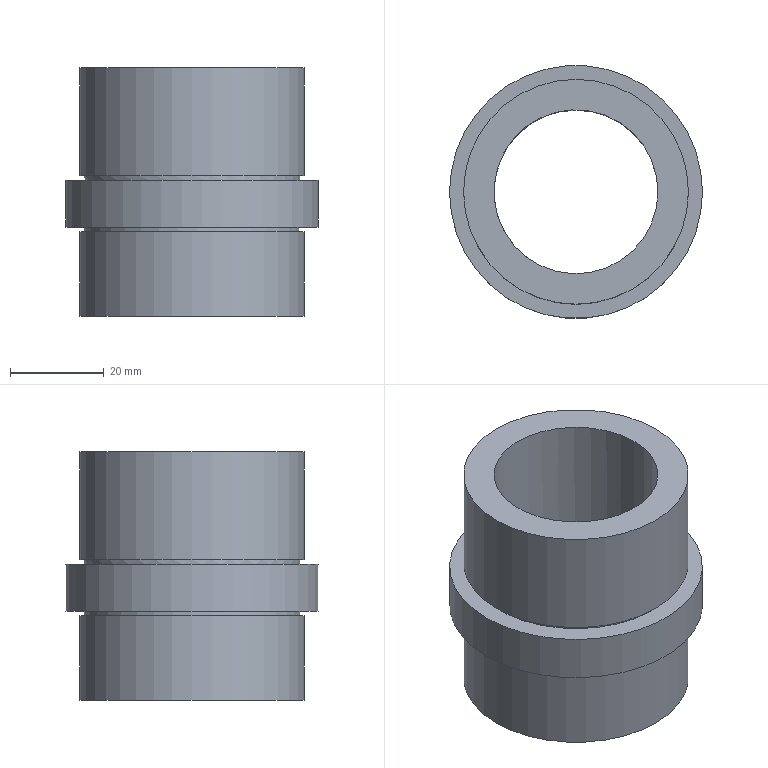Part | STEP file | 车灯-后视镜_id30_x_t | 1 solid | 12 faces | box 54 x 54 x 53 mm | volume 49426 mm3 | cylinder 6 | plane 6 | commonest cylinder face diameters 46 x2 48 x2 35 x1 54 x1
STEP:
#1=CARTESIAN_POINT('',(86.,185.,-254.5));
#2=VERTEX_POINT('',#1);
#3=CARTESIAN_POINT('',(110.,185.,-254.5));
#4=DIRECTION('',(0.,0.,1.));
#5=DIRECTION('',(-1.,0.,0.));
#6=AXIS2_PLACEMENT_3D('',#3,#4,#5);
#7=CIRCLE('',#6,24.);
#8=EDGE_CURVE('',#2,#2,#7,.T.);
#9=ORIENTED_EDGE('',*,*,#8,.T.);
#10=EDGE_LOOP('',(#9));
#11=FACE_BOUND('',#10,.T.);
#12=CARTESIAN_POINT('',(86.,185.,-231.5));
#13=VERTEX_POINT('',#12);
#14=CARTESIAN_POINT('',(110.,185.,-231.5));
#15=DIRECTION('',(0.,0.,1.));
#16=DIRECTION('',(-1.,0.,0.));
#17=AXIS2_PLACEMENT_3D('',#14,#15,#16);
#18=CIRCLE('',#17,24.);
#19=EDGE_CURVE('',#13,#13,#18,.T.);
#20=ORIENTED_EDGE('',*,*,#19,.F.);
#21=EDGE_LOOP('',(#20));
#22=FACE_BOUND('',#21,.T.);
#23=CARTESIAN_POINT('',(110.,185.,-284.5));
#24=DIRECTION('',(0.,0.,1.));
#25=DIRECTION('',(1.,0.,0.));
#26=AXIS2_PLACEMENT_3D('',#23,#24,#25);
#27=CYLINDRICAL_SURFACE('',#26,24.);
#28=ADVANCED_FACE('',(#11,#22),#27,.T.);
#29=CARTESIAN_POINT('',(127.5,185.,-231.5));
#30=VERTEX_POINT('',#29);
#31=CARTESIAN_POINT('',(110.,185.,-231.5));
#32=DIRECTION('',(0.,0.,-1.));
#33=DIRECTION('',(1.,0.,0.));
#34=AXIS2_PLACEMENT_3D('',#31,#32,#33);
#35=CIRCLE('',#34,17.5);
#36=EDGE_CURVE('',#30,#30,#35,.T.);
#37=ORIENTED_EDGE('',*,*,#36,.T.);
#38=EDGE_LOOP('',(#37));
#39=FACE_BOUND('',#38,.T.);
#40=ORIENTED_EDGE('',*,*,#19,.T.);
#41=EDGE_LOOP('',(#40));
#42=FACE_BOUND('',#41,.T.);
#43=CARTESIAN_POINT('',(110.,185.,-231.5));
#44=DIRECTION('',(0.,0.,1.));
#45=DIRECTION('',(1.,0.,0.));
#46=AXIS2_PLACEMENT_3D('',#43,#44,#45);
#47=PLANE('',#46);
#48=ADVANCED_FACE('',(#39,#42),#47,.T.);
#49=ORIENTED_EDGE('',*,*,#36,.F.);
#50=EDGE_LOOP('',(#49));
#51=FACE_BOUND('',#50,.T.);
#52=CARTESIAN_POINT('',(92.5,185.,-284.5));
#53=VERTEX_POINT('',#52);
#54=CARTESIAN_POINT('',(110.,185.,-284.5));
#55=DIRECTION('',(0.,0.,1.));
#56=DIRECTION('',(-1.,0.,0.));
#57=AXIS2_PLACEMENT_3D('',#54,#55,#56);
#58=CIRCLE('',#57,17.5);
#59=EDGE_CURVE('',#53,#53,#58,.T.);
#60=ORIENTED_EDGE('',*,*,#59,.F.);
#61=EDGE_LOOP('',(#60));
#62=FACE_BOUND('',#61,.T.);
#63=CARTESIAN_POINT('',(110.,185.,-285.5));
#64=DIRECTION('',(0.,0.,1.));
#65=DIRECTION('',(1.,0.,0.));
#66=AXIS2_PLACEMENT_3D('',#63,#64,#65);
#67=CYLINDRICAL_SURFACE('',#66,17.5);
#68=ADVANCED_FACE('',(#51,#62),#67,.F.);
#69=CARTESIAN_POINT('',(87.,185.,-254.5));
#70=VERTEX_POINT('',#69);
#71=CARTESIAN_POINT('',(110.,185.,-254.5));
#72=DIRECTION('',(0.,0.,1.));
#73=DIRECTION('',(-1.,0.,0.));
#74=AXIS2_PLACEMENT_3D('',#71,#72,#73);
#75=CIRCLE('',#74,23.);
#76=EDGE_CURVE('',#70,#70,#75,.T.);
#77=ORIENTED_EDGE('',*,*,#76,.T.);
#78=EDGE_LOOP('',(#77));
#79=FACE_BOUND('',#78,.T.);
#80=ORIENTED_EDGE('',*,*,#8,.F.);
#81=EDGE_LOOP('',(#80));
#82=FACE_BOUND('',#81,.T.);
#83=CARTESIAN_POINT('',(110.,185.,-254.5));
#84=DIRECTION('',(0.,0.,1.));
#85=DIRECTION('',(1.,0.,0.));
#86=AXIS2_PLACEMENT_3D('',#83,#84,#85);
#87=PLANE('',#86);
#88=ADVANCED_FACE('',(#79,#82),#87,.F.);
#89=ORIENTED_EDGE('',*,*,#76,.F.);
#90=EDGE_LOOP('',(#89));
#91=FACE_BOUND('',#90,.T.);
#92=CARTESIAN_POINT('',(133.,185.,-255.5));
#93=VERTEX_POINT('',#92);
#94=CARTESIAN_POINT('',(110.,185.,-255.5));
#95=DIRECTION('',(0.,0.,1.));
#96=DIRECTION('',(1.,0.,0.));
#97=AXIS2_PLACEMENT_3D('',#94,#95,#96);
#98=CIRCLE('',#97,23.);
#99=EDGE_CURVE('',#93,#93,#98,.T.);
#100=ORIENTED_EDGE('',*,*,#99,.T.);
#101=EDGE_LOOP('',(#100));
#102=FACE_BOUND('',#101,.T.);
#103=CARTESIAN_POINT('',(110.,185.,-255.5));
#104=DIRECTION('',(0.,0.,1.));
#105=DIRECTION('',(1.,0.,0.));
#106=AXIS2_PLACEMENT_3D('',#103,#104,#105);
#107=CYLINDRICAL_SURFACE('',#106,23.);
#108=ADVANCED_FACE('',(#91,#102),#107,.T.);
#109=CARTESIAN_POINT('',(87.,185.,-265.5));
#110=VERTEX_POINT('',#109);
#111=CARTESIAN_POINT('',(110.,185.,-265.5));
#112=DIRECTION('',(0.,0.,1.));
#113=DIRECTION('',(-1.,0.,0.));
#114=AXIS2_PLACEMENT_3D('',#111,#112,#113);
#115=CIRCLE('',#114,23.);
#116=EDGE_CURVE('',#110,#110,#115,.T.);
#117=ORIENTED_EDGE('',*,*,#116,.T.);
#118=EDGE_LOOP('',(#117));
#119=FACE_BOUND('',#118,.T.);
#120=CARTESIAN_POINT('',(137.,185.,-265.5));
#121=VERTEX_POINT('',#120);
#122=CARTESIAN_POINT('',(110.,185.,-265.5));
#123=DIRECTION('',(0.,0.,-1.));
#124=DIRECTION('',(1.,0.,0.));
#125=AXIS2_PLACEMENT_3D('',#122,#123,#124);
#126=CIRCLE('',#125,27.);
#127=EDGE_CURVE('',#121,#121,#126,.T.);
#128=ORIENTED_EDGE('',*,*,#127,.T.);
#129=EDGE_LOOP('',(#128));
#130=FACE_BOUND('',#129,.T.);
#131=CARTESIAN_POINT('',(110.,185.,-265.5));
#132=DIRECTION('',(0.,0.,-1.));
#133=DIRECTION('',(-1.,0.,0.));
#134=AXIS2_PLACEMENT_3D('',#131,#132,#133);
#135=PLANE('',#134);
#136=ADVANCED_FACE('',(#119,#130),#135,.T.);
#137=ORIENTED_EDGE('',*,*,#99,.F.);
#138=EDGE_LOOP('',(#137));
#139=FACE_BOUND('',#138,.T.);
#140=CARTESIAN_POINT('',(83.,185.,-255.5));
#141=VERTEX_POINT('',#140);
#142=CARTESIAN_POINT('',(110.,185.,-255.5));
#143=DIRECTION('',(0.,0.,1.));
#144=DIRECTION('',(-1.,0.,0.));
#145=AXIS2_PLACEMENT_3D('',#142,#143,#144);
#146=CIRCLE('',#145,27.);
#147=EDGE_CURVE('',#141,#141,#146,.T.);
#148=ORIENTED_EDGE('',*,*,#147,.T.);
#149=EDGE_LOOP('',(#148));
#150=FACE_BOUND('',#149,.T.);
#151=CARTESIAN_POINT('',(110.,185.,-255.5));
#152=DIRECTION('',(0.,0.,1.));
#153=DIRECTION('',(1.,0.,0.));
#154=AXIS2_PLACEMENT_3D('',#151,#152,#153);
#155=PLANE('',#154);
#156=ADVANCED_FACE('',(#139,#150),#155,.T.);
#157=ORIENTED_EDGE('',*,*,#127,.F.);
#158=EDGE_LOOP('',(#157));
#159=FACE_BOUND('',#158,.T.);
#160=ORIENTED_EDGE('',*,*,#147,.F.);
#161=EDGE_LOOP('',(#160));
#162=FACE_BOUND('',#161,.T.);
#163=CARTESIAN_POINT('',(110.,185.,-255.5));
#164=DIRECTION('',(0.,0.,-1.));
#165=DIRECTION('',(-1.,0.,0.));
#166=AXIS2_PLACEMENT_3D('',#163,#164,#165);
#167=CYLINDRICAL_SURFACE('',#166,27.);
#168=ADVANCED_FACE('',(#159,#162),#167,.T.);
#169=ORIENTED_EDGE('',*,*,#116,.F.);
#170=EDGE_LOOP('',(#169));
#171=FACE_BOUND('',#170,.T.);
#172=CARTESIAN_POINT('',(87.,185.,-266.5));
#173=VERTEX_POINT('',#172);
#174=CARTESIAN_POINT('',(110.,185.,-266.5));
#175=DIRECTION('',(0.,0.,-1.));
#176=DIRECTION('',(-1.,0.,0.));
#177=AXIS2_PLACEMENT_3D('',#174,#175,#176);
#178=CIRCLE('',#177,23.);
#179=EDGE_CURVE('',#173,#173,#178,.T.);
#180=ORIENTED_EDGE('',*,*,#179,.F.);
#181=EDGE_LOOP('',(#180));
#182=FACE_BOUND('',#181,.T.);
#183=CARTESIAN_POINT('',(110.,185.,-266.5));
#184=DIRECTION('',(0.,0.,1.));
#185=DIRECTION('',(1.,0.,0.));
#186=AXIS2_PLACEMENT_3D('',#183,#184,#185);
#187=CYLINDRICAL_SURFACE('',#186,23.);
#188=ADVANCED_FACE('',(#171,#182),#187,.T.);
#189=CARTESIAN_POINT('',(134.,185.,-266.5));
#190=VERTEX_POINT('',#189);
#191=CARTESIAN_POINT('',(110.,185.,-266.5));
#192=DIRECTION('',(0.,0.,-1.));
#193=DIRECTION('',(1.,0.,0.));
#194=AXIS2_PLACEMENT_3D('',#191,#192,#193);
#195=CIRCLE('',#194,24.);
#196=EDGE_CURVE('',#190,#190,#195,.T.);
#197=ORIENTED_EDGE('',*,*,#196,.T.);
#198=EDGE_LOOP('',(#197));
#199=FACE_BOUND('',#198,.T.);
#200=CARTESIAN_POINT('',(134.,185.,-284.5));
#201=VERTEX_POINT('',#200);
#202=CARTESIAN_POINT('',(110.,185.,-284.5));
#203=DIRECTION('',(0.,0.,-1.));
#204=DIRECTION('',(1.,0.,0.));
#205=AXIS2_PLACEMENT_3D('',#202,#203,#204);
#206=CIRCLE('',#205,24.);
#207=EDGE_CURVE('',#201,#201,#206,.T.);
#208=ORIENTED_EDGE('',*,*,#207,.F.);
#209=EDGE_LOOP('',(#208));
#210=FACE_BOUND('',#209,.T.);
#211=CARTESIAN_POINT('',(110.,185.,-284.5));
#212=DIRECTION('',(0.,0.,1.));
#213=DIRECTION('',(1.,0.,0.));
#214=AXIS2_PLACEMENT_3D('',#211,#212,#213);
#215=CYLINDRICAL_SURFACE('',#214,24.);
#216=ADVANCED_FACE('',(#199,#210),#215,.T.);
#217=ORIENTED_EDGE('',*,*,#59,.T.);
#218=EDGE_LOOP('',(#217));
#219=FACE_BOUND('',#218,.T.);
#220=ORIENTED_EDGE('',*,*,#207,.T.);
#221=EDGE_LOOP('',(#220));
#222=FACE_BOUND('',#221,.T.);
#223=CARTESIAN_POINT('',(110.,185.,-284.5));
#224=DIRECTION('',(0.,0.,-1.));
#225=DIRECTION('',(-1.,0.,0.));
#226=AXIS2_PLACEMENT_3D('',#223,#224,#225);
#227=PLANE('',#226);
#228=ADVANCED_FACE('',(#219,#222),#227,.T.);
#229=ORIENTED_EDGE('',*,*,#179,.T.);
#230=EDGE_LOOP('',(#229));
#231=FACE_BOUND('',#230,.T.);
#232=ORIENTED_EDGE('',*,*,#196,.F.);
#233=EDGE_LOOP('',(#232));
#234=FACE_BOUND('',#233,.T.);
#235=CARTESIAN_POINT('',(110.,185.,-266.5));
#236=DIRECTION('',(0.,0.,-1.));
#237=DIRECTION('',(-1.,0.,0.));
#238=AXIS2_PLACEMENT_3D('',#235,#236,#237);
#239=PLANE('',#238);
#240=ADVANCED_FACE('',(#231,#234),#239,.F.);
#241=CLOSED_SHELL('',(#28,#48,#68,#88,#108,#136,#156,#168,#188,#216,#228,#240));
#242=MANIFOLD_SOLID_BREP('',#241);
#243=(LENGTH_UNIT()NAMED_UNIT(*)SI_UNIT(.MILLI.,.METRE.));
#244=UNCERTAINTY_MEASURE_WITH_UNIT(LENGTH_MEASURE(0.00002),#243,'','');
#245=(NAMED_UNIT(*)PLANE_ANGLE_UNIT()SI_UNIT($,.RADIAN.));
#246=PLANE_ANGLE_MEASURE_WITH_UNIT(PLANE_ANGLE_MEASURE(0.01745),#245);
#247=DIMENSIONAL_EXPONENTS(0.,0.,0.,0.,0.,0.,0.);
#248=(CONVERSION_BASED_UNIT('DEGREE',#246)NAMED_UNIT(#247)PLANE_ANGLE_UNIT());
#249=(NAMED_UNIT(*)SI_UNIT($,.STERADIAN.)SOLID_ANGLE_UNIT());
#250=(GEOMETRIC_REPRESENTATION_CONTEXT(3)GLOBAL_UNCERTAINTY_ASSIGNED_CONTEXT((#244))GLOBAL_UNIT_ASSIGNED_CONTEXT((#243,#248,#249))REPRESENTATION_CONTEXT('',''));
#251=ADVANCED_BREP_SHAPE_REPRESENTATION('',(#242),#250);